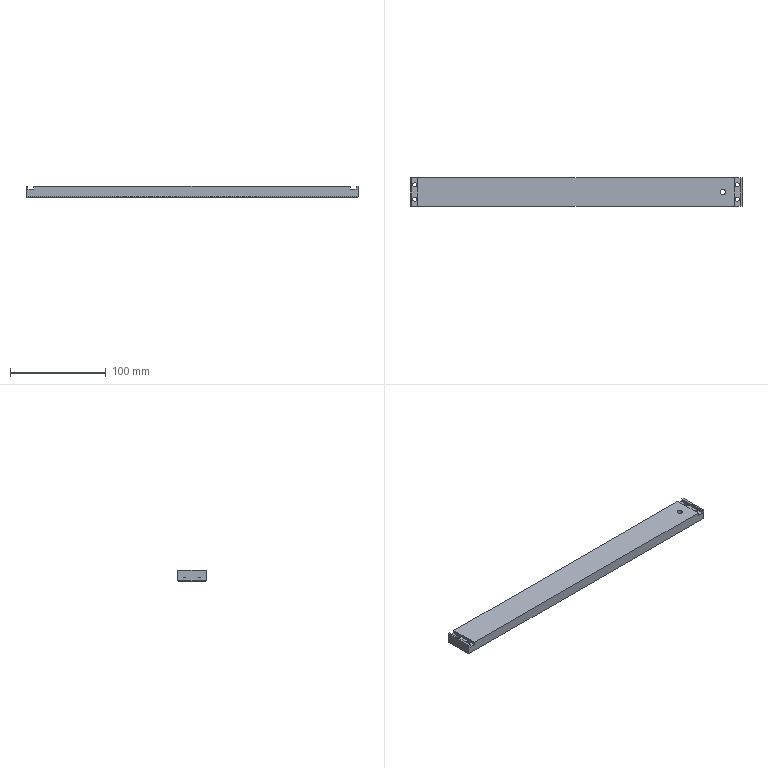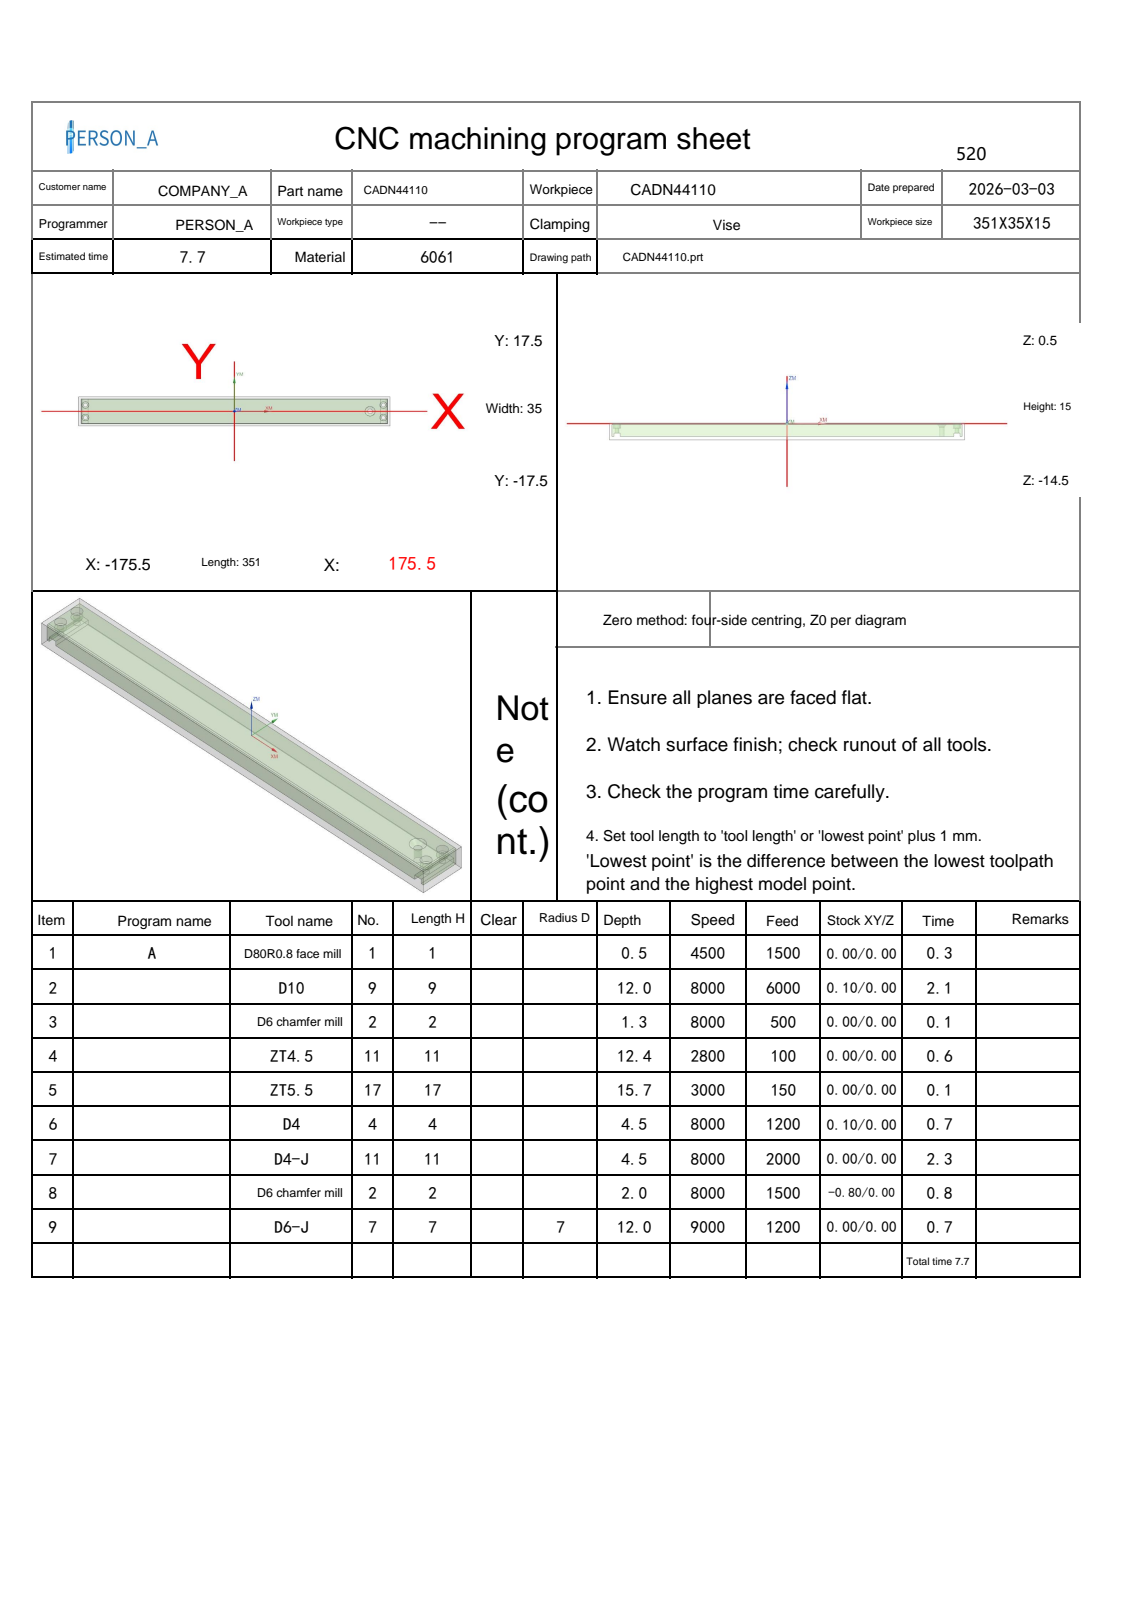NC program | NX | posted by the shop | part box 346 x 30 x 11.5 mm
Lines 337 to 1758 of 28539:
N7 T11 M06
(D4-J  D=4. R=0. H=11 ce=0.01 di=0.00)
G00 G90 G54 X149.305 Y-.481 M03 S7000
G43 H11 Z30.
M08
Z1.5
G01 X149.362 Y-.844 Z1.481 F2000.
X149.522 Y-1.359 Z1.452
X149.754 Y-1.846 Z1.424
X150.053 Y-2.294 Z1.396
X150.414 Y-2.695 Z1.368
X150.829 Y-3.039 Z1.339
X151.29 Y-3.32 Z1.311
X151.786 Y-3.531 Z1.283
X152.157 Y-3.638 Z1.263
X152.48 Y-3.698 Z1.245
X152.807 Y-3.729 Z1.228
X153.193 Z1.208
X153.206 Z1.207
X153.59 Y-3.687 Z1.187
X154.09 Y-3.572 Z1.16
X154.569 Y-3.389 Z1.133
X155.018 Y-3.142 Z1.106
X155.43 Y-2.836 Z1.08
X155.795 Y-2.477 Z1.053
X156.108 Y-2.07 Z1.026
X156.362 Y-1.625 Z.999
X156.553 Y-1.149 Z.972
X156.677 Y-.652 Z.945
X156.732 Y-.142 Z.918
X156.716 Y.37 Z.892
X156.63 Y.876 Z.865
X156.476 Y1.365 Z.838
X156.256 Y1.828 Z.811
X156.05 Y2.155 Z.791
X155.725 Y2.553 Z.764
X155.349 Y2.903 Z.737
X154.928 Y3.198 Z.71
X154.471 Y3.433 Z.683
X153.985 Y3.602 Z.656
X153.481 Y3.703 Z.629
X152.968 Y3.734 Z.602
X152.456 Y3.695 Z.575
X151.954 Y3.585 Z.548
X151.472 Y3.407 Z.521
X151.018 Y3.165 Z.494
X150.602 Y2.863 Z.467
X150.232 Y2.507 Z.44
X149.914 Y2.103 Z.414
X149.713 Y1.773 Z.393
X149.492 Y1.281 Z.365
X149.344 Y.762 Z.337
X149.273 Y.228 Z.309
X149.279 Y-.311 Z.28
X149.362 Y-.844 Z.252
X149.522 Y-1.359 Z.224
X149.754 Y-1.846 Z.195
X150.053 Y-2.294 Z.167
X150.414 Y-2.695 Z.139
X150.829 Y-3.039 Z.111
X151.29 Y-3.32 Z.082
X151.786 Y-3.531 Z.054
X152.157 Y-3.638 Z.034
X152.48 Y-3.698 Z.017
X152.807 Y-3.729 Z0.0
X153. Z-.011
G03 X156.729 Y0.0 I0.0 J3.729
X153. Y3.729 I-3.729 J0.0
X149.271 Y0.0 I0.0 J-3.729
X153. Y-3.729 I3.729 J0.0
G01 X153.1 Y-3.728
X153.199 Y-3.724
X153.3 Y-3.717
X153.399 Y-3.708
X153.586 Y-3.683
X153.771 Y-3.648
X153.955 Y-3.605
X154.137 Y-3.551
X154.315 Y-3.489
X154.49 Y-3.418
X154.661 Y-3.338
X154.828 Y-3.25
X154.99 Y-3.153 Z-.012
X155.147 Y-3.048
X155.299 Y-2.935
X155.445 Y-2.815
X155.584 Y-2.687
X155.717 Y-2.553
X155.843 Y-2.412
X155.961 Y-2.265
X156.072 Y-2.112
X156.175 Y-1.953
X156.27 Y-1.79
X156.356 Y-1.622 Z-.013
X156.434 Y-1.45
X156.503 Y-1.274
X156.563 Y-1.095
X156.614 Y-.913
X156.655 Y-.729
X156.687 Y-.543
X156.71 Y-.355
X156.723 Y-.167
X156.727 Y.022
X156.721 Y.211
X156.705 Y.399
X156.68 Y.586 Z-.014
X156.646 Y.772
X156.602 Y.955
X156.549 Y1.136
X156.486 Y1.315
X156.415 Y1.49
X156.335 Y1.661
X156.247 Y1.827
X156.15 Y1.99
X156.045 Y2.147
X155.932 Y2.299
X155.811 Y2.445
X155.684 Y2.584 Z-.015
X155.549 Y2.717
X155.408 Y2.843
X155.26 Y2.961
X155.107 Y3.072
X154.948 Y3.175
X154.784 Y3.27
X154.616 Y3.356
X154.443 Y3.434
X154.267 Y3.503
X154.088 Y3.562
X153.905 Y3.613 Z-.016
X153.721 Y3.654
X153.534 Y3.686
X153.346 Y3.708
X153.158 Y3.721
X152.968 Y3.724
X152.779 Y3.717
X152.591 Y3.701
X152.404 Y3.676
X152.218 Y3.641
X152.034 Y3.596
X151.853 Y3.542
X151.674 Y3.479 Z-.017
X151.499 Y3.408
X151.328 Y3.327
X151.162 Y3.238
X151. Y3.14
X150.843 Y3.034
X150.692 Y2.921
X150.546 Y2.8
X150.407 Y2.672
X150.275 Y2.536
X150.15 Y2.395
X150.032 Y2.247
X149.942 Y2.122 Z-.018
X149.856 Y1.993
X149.838 Y1.964
X149.82 Y1.934
X149.725 Y1.769
X149.639 Y1.6
X149.562 Y1.426
X149.494 Y1.249
X149.435 Y1.068
X149.385 Y.885
X149.345 Y.699
X149.314 Y.512
X149.292 Y.323
X149.281 Y.134 Z-.019
X149.279 Y-.056
X149.287 Y-.246
X149.304 Y-.435
X149.331 Y-.623
X149.368 Y-.81
X149.414 Y-.994
X149.47 Y-1.176
X149.534 Y-1.354
X149.608 Y-1.529
X149.691 Y-1.7
X149.782 Y-1.867
X149.881 Y-2.029 Z-.02
X149.989 Y-2.185
X150.104 Y-2.336
X150.227 Y-2.48
X150.358 Y-2.619
X150.495 Y-2.75
X150.638 Y-2.874
X150.788 Y-2.991
X150.944 Y-3.1
X151.105 Y-3.201
X151.27 Y-3.293
X151.441 Y-3.377
X151.615 Y-3.452 Z-.021
X151.793 Y-3.518
X151.974 Y-3.575
X151.992 Y-3.58
X152.01 Y-3.585
X152.16 Y-3.623
X152.311 Y-3.655
X152.482 Y-3.683
X152.654 Y-3.703
X152.827 Y-3.715
X153. Y-3.719
X153.1 Y-3.717
X153.199 Y-3.713
X153.3 Y-3.707
X153.399 Y-3.697
X153.586 Y-3.672
X153.771 Y-3.638 Z-.022
X153.954 Y-3.594
X154.135 Y-3.541
X154.313 Y-3.479
X154.488 Y-3.408
X154.658 Y-3.328
X154.825 Y-3.239
X154.987 Y-3.143
X155.143 Y-3.038
X155.295 Y-2.925
X155.44 Y-2.805
X155.579 Y-2.678 Z-.023
X155.711 Y-2.543
X155.837 Y-2.403
X155.955 Y-2.256
X156.065 Y-2.103
X156.168 Y-1.945
X156.262 Y-1.782
X156.348 Y-1.614
X156.426 Y-1.442
X156.494 Y-1.267
X156.554 Y-1.088
X156.604 Y-.906
X156.646 Y-.722 Z-.024
X156.677 Y-.537
X156.7 Y-.349
X156.713 Y-.161
X156.716 Y.027
X156.71 Y.215
X156.694 Y.403
X156.669 Y.59
X156.634 Y.775
X156.59 Y.958
X156.537 Y1.139
X156.474 Y1.317
X156.403 Y1.491 Z-.025
X156.323 Y1.662
X156.234 Y1.828
X156.138 Y1.99
X156.034 Y2.145
X155.922 Y2.294
X155.803 Y2.438
X155.677 Y2.576
X155.544 Y2.707
X155.404 Y2.832
X155.259 Y2.949
X155.108 Y3.059 Z-.026
X154.951 Y3.161
X154.79 Y3.255
X154.624 Y3.34
X154.454 Y3.418
X154.28 Y3.486
X154.104 Y3.546
X153.924 Y3.597
X153.742 Y3.639
X153.558 Y3.672
X153.373 Y3.695
X153.187 Y3.709
X153. Y3.713 Z-.027
X152.813 Y3.709
X152.627 Y3.695
X152.442 Y3.671
X152.258 Y3.638
X152.076 Y3.596
X151.897 Y3.545
X151.72 Y3.485
X151.546 Y3.416
X151.377 Y3.339
X151.211 Y3.253
X151.05 Y3.159
X150.893 Y3.057 Z-.028
X150.742 Y2.947
X150.597 Y2.83
X150.458 Y2.705
X150.325 Y2.574
X150.199 Y2.436
X150.081 Y2.293
X149.969 Y2.143
X149.865 Y1.988
X149.767 Y1.823
X149.677 Y1.653
X149.595 Y1.478
X149.524 Y1.3 Z-.029
X149.461 Y1.118
X149.408 Y.933
X149.364 Y.745
X149.331 Y.556
X149.307 Y.365
X149.293 Y.173
X149.289 Y-.019
X149.295 Y-.212
X149.311 Y-.403
X149.337 Y-.594
X149.373 Y-.783 Z-.03
X149.419 Y-.97
X149.474 Y-1.154
X149.538 Y-1.335
X149.612 Y-1.513
X149.695 Y-1.686
X149.787 Y-1.855
X149.888 Y-2.019
X149.997 Y-2.178
X150.114 Y-2.33
X150.238 Y-2.477
X150.371 Y-2.617
X150.51 Y-2.749 Z-.031
X150.656 Y-2.875
X150.808 Y-2.992
X150.966 Y-3.102
X151.129 Y-3.203
X151.298 Y-3.295
X151.471 Y-3.379
X151.648 Y-3.454
X151.829 Y-3.519
X152.013 Y-3.575
X152.032 Y-3.58
X152.051 Y-3.585
X152.194 Y-3.62
X152.338 Y-3.649 Z-.032
X152.502 Y-3.675
X152.668 Y-3.693
X152.834 Y-3.705
X153. Y-3.708
X153.1 Y-3.707
X153.199 Y-3.703
X153.3 Y-3.696
X153.399 Y-3.686
X153.585 Y-3.661
X153.77 Y-3.627
X153.953 Y-3.583
X154.133 Y-3.53
X154.311 Y-3.468
X154.485 Y-3.397 Z-.033
X154.655 Y-3.317
X154.822 Y-3.229
X154.983 Y-3.132
X155.139 Y-3.028
X155.29 Y-2.915
X155.435 Y-2.795
X155.574 Y-2.668
X155.706 Y-2.534
X155.831 Y-2.393
X155.948 Y-2.247
X156.058 Y-2.094
X156.161 Y-1.936 Z-.034
X156.255 Y-1.773
X156.34 Y-1.606
X156.417 Y-1.434
X156.486 Y-1.259
X156.545 Y-1.081
X156.595 Y-.899
X156.636 Y-.716
X156.668 Y-.53
X156.69 Y-.344
X156.702 Y-.156
X156.705 Y.032
X156.699 Y.22 Z-.035
X156.683 Y.407
X156.657 Y.594
X156.622 Y.778
X156.578 Y.961
X156.525 Y1.141
X156.462 Y1.319
X156.391 Y1.493
X156.311 Y1.663
X156.222 Y1.829
X156.125 Y1.99
X156.021 Y2.144 Z-.036
X155.91 Y2.293
X155.791 Y2.436
X155.665 Y2.573
X155.533 Y2.703
X155.394 Y2.827
X155.249 Y2.943
X155.098 Y3.052
X154.943 Y3.153
X154.782 Y3.247
X154.617 Y3.332
X154.447 Y3.409
X154.275 Y3.477 Z-.037
X154.099 Y3.537
X153.92 Y3.587
X153.739 Y3.629
X153.556 Y3.661
X153.371 Y3.684
X153.186 Y3.698
X153. Y3.703
X152.814 Y3.698
X152.629 Y3.684
X152.445 Y3.661
X152.262 Y3.628
X152.081 Y3.586 Z-.038
X151.902 Y3.536
X151.726 Y3.476
X151.553 Y3.408
X151.384 Y3.331
X151.219 Y3.245
X151.058 Y3.152
X150.903 Y3.05
X150.752 Y2.941
X150.608 Y2.825
X150.469 Y2.701
X150.337 Y2.571
X150.211 Y2.434 Z-.039
X150.093 Y2.291
X149.981 Y2.142
X149.878 Y1.988
X149.784 Y1.831
X149.697 Y1.67
X149.619 Y1.504
X149.548 Y1.335
X149.487 Y1.163
X149.434 Y.988
X149.389 Y.811
X149.354 Y.631
X149.327 Y.45 Z-.04
X149.309 Y.268
X149.301 Y.085
Y-.098
X149.311 Y-.28
X149.329 Y-.462
X149.356 Y-.643
X149.393 Y-.823
X149.438 Y-1.
X149.492 Y-1.175
X149.554 Y-1.347
X149.625 Y-1.515
X149.704 Y-1.68 Z-.041
X149.791 Y-1.841
X149.886 Y-1.997
X149.989 Y-2.149
X150.099 Y-2.295
X150.216 Y-2.435
X150.34 Y-2.57
X150.47 Y-2.698
X150.606 Y-2.82
X150.749 Y-2.935
X150.897 Y-3.042
X151.05 Y-3.142
X151.207 Y-3.235 Z-.042
X151.37 Y-3.32
X151.536 Y-3.396
X151.705 Y-3.464
X151.878 Y-3.524
X152.054 Y-3.575
X152.073 Y-3.58
X152.093 Y-3.585
X152.229 Y-3.617
X152.365 Y-3.643
X152.523 Y-3.667
X152.681 Y-3.684
X152.841 Y-3.694
X153. Y-3.698
X153.1 Y-3.696
X153.199 Y-3.692 Z-.043
X153.299 Y-3.685
X153.398 Y-3.676
X153.499 Y-3.664
X153.599 Y-3.648
X153.684 Y-3.633
X153.769 Y-3.616
X153.952 Y-3.573
X154.132 Y-3.52
X154.309 Y-3.458
X154.483 Y-3.387
X154.653 Y-3.307
X154.818 Y-3.219
X154.979 Y-3.122
X155.135 Y-3.017
X155.286 Y-2.905 Z-.044
X155.43 Y-2.785
X155.568 Y-2.658
X155.7 Y-2.524
X155.825 Y-2.384
X155.942 Y-2.237
X156.052 Y-2.085
X156.153 Y-1.927
X156.247 Y-1.765
X156.332 Y-1.598
X156.409 Y-1.426
X156.477 Y-1.251
X156.536 Y-1.073 Z-.045
X156.586 Y-.892
X156.627 Y-.709
X156.658 Y-.524
X156.68 Y-.338
X156.692 Y-.15
X156.695 Y.037
X156.688 Y.225
X156.672 Y.412
X156.646 Y.598
X156.611 Y.782
X156.566 Y.964 Z-.046
X156.513 Y1.144
X156.45 Y1.321
X156.379 Y1.494
X156.298 Y1.664
X156.209 Y1.829
X156.112 Y1.99
X156.009 Y2.143
X155.898 Y2.291
X155.779 Y2.433
X155.654 Y2.569
X155.522 Y2.699
X155.383 Y2.822 Z-.047
X155.239 Y2.937
X155.089 Y3.046
X154.934 Y3.146
X154.774 Y3.239
X154.609 Y3.324
X154.441 Y3.4
X154.269 Y3.468
X154.093 Y3.527
X153.915 Y3.577
X153.735 Y3.619
X153.553 Y3.651
X153.369 Y3.674 Z-.048
X153.185 Y3.688
X153. Y3.692
X152.815 Y3.688
X152.631 Y3.674
X152.447 Y3.65
X152.265 Y3.618
X152.085 Y3.577
X151.907 Y3.526
X151.732 Y3.467
X151.56 Y3.399
X151.391 Y3.323
X151.227 Y3.238 Z-.049
X151.067 Y3.145
X150.912 Y3.044
X150.762 Y2.936
X150.618 Y2.82
X150.48 Y2.697
X150.348 Y2.567
X150.223 Y2.431
X150.105 Y2.289
X149.994 Y2.141
X149.89 Y1.988
X149.795 Y1.83 Z-.05
X149.708 Y1.669
X149.63 Y1.503
X149.559 Y1.333
X149.497 Y1.16
X149.444 Y.984
X149.399 Y.806
X149.364 Y.626
X149.337 Y.444
X149.32 Y.261
X149.311 Y.078
X149.312 Y-.106
X149.322 Y-.289 Z-.051
X149.341 Y-.472
X149.369 Y-.653
X149.406 Y-.833
X149.452 Y-1.011
X149.507 Y-1.186
X149.57 Y-1.359
X149.642 Y-1.528
X149.722 Y-1.693
X149.811 Y-1.854
X149.907 Y-2.01
X150.011 Y-2.161
X150.122 Y-2.307 Z-.052
X150.241 Y-2.448
X150.366 Y-2.582
X150.498 Y-2.71
X150.636 Y-2.831
X150.78 Y-2.945
X150.929 Y-3.052
X151.084 Y-3.151
X151.243 Y-3.242
X151.406 Y-3.326
X151.574 Y-3.401
X151.745 Y-3.467
X151.919 Y-3.525 Z-.053
X152.096 Y-3.575
X152.117 Y-3.58
X152.138 Y-3.585
X152.265 Y-3.613
X152.394 Y-3.637
X152.544 Y-3.659
X152.696 Y-3.675
X152.848 Y-3.684
X153. Y-3.687
X153.15 Y-3.684
X153.3 Y-3.675
X153.45 Y-3.659
X153.599 Y-3.638
X153.787 Y-3.602
X153.972 Y-3.556
X154.156 Y-3.5 Z-.054
X154.337 Y-3.435
X154.514 Y-3.361
X154.686 Y-3.278
X154.855 Y-3.185
X155.018 Y-3.085
X155.176 Y-2.975
X155.328 Y-2.858
X155.473 Y-2.733
X155.612 Y-2.6
X155.744 Y-2.461
X155.868 Y-2.315 Z-.055
X155.984 Y-2.162
X156.093 Y-2.004
X156.193 Y-1.84
X156.284 Y-1.671
X156.367 Y-1.498
X156.44 Y-1.321
X156.504 Y-1.14
X156.559 Y-.956
X156.603 Y-.77
X156.638 Y-.581
X156.664 Y-.391 Z-.056
X156.679 Y-.2
X156.684 Y-.008
X156.68 Y.184
X156.665 Y.375
X156.64 Y.565
X156.606 Y.754
X156.562 Y.941
X156.508 Y1.125
X156.445 Y1.306
X156.372 Y1.483
X156.29 Y1.657
X156.199 Y1.826 Z-.057
X156.1 Y1.99
X155.996 Y2.142
X155.886 Y2.289
X155.767 Y2.43
X155.642 Y2.566
X155.511 Y2.694
X155.373 Y2.816
X155.229 Y2.932
X155.08 Y3.039
X154.925 Y3.139
X154.766 Y3.232
X154.602 Y3.316 Z-.058
X154.434 Y3.392
X154.263 Y3.459
X154.088 Y3.518
X153.911 Y3.568
X153.732 Y3.609
X153.55 Y3.641
X153.368 Y3.663
X153.184 Y3.677
X153. Y3.682
X152.816 Y3.677
X152.632 Y3.663 Z-.059
X152.45 Y3.64
X152.269 Y3.608
X152.089 Y3.567
X151.912 Y3.517
X151.738 Y3.458
X151.566 Y3.39
X151.399 Y3.314
X151.235 Y3.23
X151.076 Y3.138
X150.921 Y3.038
X150.772 Y2.93
X150.629 Y2.815 Z-.06
X150.491 Y2.693
X150.36 Y2.564
X150.235 Y2.428
X150.117 Y2.287
X150.006 Y2.14
X149.903 Y1.988
X149.807 Y1.83
X149.72 Y1.668
X149.64 Y1.501
X149.569 Y1.331
X149.507 Y1.157
X149.454 Y.981 Z-.061
X149.409 Y.802
X149.373 Y.621
X149.347 Y.438
X149.33 Y.254
X149.322 Y.07
X149.323 Y-.114
X149.333 Y-.298
X149.353 Y-.482
X149.382 Y-.664
X149.42 Y-.845
X149.467 Y-1.023
X149.522 Y-1.199 Z-.062
X149.587 Y-1.371
X149.66 Y-1.541
X149.741 Y-1.706
X149.831 Y-1.867
X149.929 Y-2.024
X150.034 Y-2.175
X150.147 Y-2.321
X150.267 Y-2.461
X150.394 Y-2.595
X150.527 Y-2.722
X150.667 Y-2.843
X150.812 Y-2.956 Z-.063
X150.963 Y-3.062
X151.119 Y-3.16
X151.28 Y-3.25
X151.445 Y-3.332
X151.614 Y-3.406
X151.786 Y-3.471
X151.962 Y-3.527
X152.14 Y-3.575
X152.162 Y-3.58
X152.184 Y-3.585
X152.304 Y-3.61
X152.424 Y-3.631
X152.567 Y-3.651
X152.711 Y-3.665 Z-.064
X152.855 Y-3.674
X153. Y-3.676
X153.15 Y-3.673
X153.3 Y-3.664
X153.45 Y-3.649
X153.599 Y-3.627
X153.786 Y-3.591
X153.971 Y-3.545
X154.155 Y-3.49
X154.335 Y-3.425
X154.511 Y-3.351
X154.684 Y-3.267
X154.852 Y-3.175 Z-.065
X155.014 Y-3.074
X155.172 Y-2.965
X155.323 Y-2.848
X155.468 Y-2.723
X155.607 Y-2.591
X155.738 Y-2.451
X155.862 Y-2.305
X155.978 Y-2.153
X156.086 Y-1.995
X156.186 Y-1.831
X156.277 Y-1.663 Z-.066
X156.359 Y-1.49
X156.432 Y-1.313
X156.495 Y-1.133
X156.549 Y-.949
X156.594 Y-.763
X156.629 Y-.575
X156.654 Y-.385
X156.669 Y-.194
X156.674 Y-.003
X156.669 Y.189
X156.654 Y.38
X156.629 Y.569 Z-.067
X156.594 Y.758
X156.55 Y.944
X156.496 Y1.127
X156.432 Y1.308
X156.36 Y1.485
X156.278 Y1.658
X156.187 Y1.826
X156.087 Y1.99
X155.984 Y2.141
X155.873 Y2.287
X155.756 Y2.428 Z-.068
X155.631 Y2.562
X155.5 Y2.69
X155.362 Y2.811
X155.219 Y2.926
X155.07 Y3.033
X154.916 Y3.132
X154.758 Y3.224
X154.595 Y3.307
X154.428 Y3.383
X154.257 Y3.45
X154.083 Y3.508
X153.907 Y3.558 Z-.069
X153.728 Y3.598
X153.548 Y3.63
X153.366 Y3.653
X153.183 Y3.667
X153. Y3.671
X152.817 Y3.666
X152.634 Y3.653
X152.452 Y3.63
X152.272 Y3.598
X152.093 Y3.557
X151.917 Y3.507
X151.743 Y3.449 Z-.07
X151.573 Y3.382
X151.406 Y3.306
X151.243 Y3.222
X151.085 Y3.131
X150.931 Y3.031
X150.782 Y2.924
X150.639 Y2.81
X150.502 Y2.688
X150.371 Y2.56
X150.247 Y2.426
X150.129 Y2.285
X150.019 Y2.139 Z-.071
X149.916 Y1.988
X149.819 Y1.829
X149.731 Y1.666
X149.651 Y1.499
X149.58 Y1.328
X149.517 Y1.154
X149.463 Y.976
X149.419 Y.797
X149.383 Y.615
X149.357 Y.431
X149.34 Y.247
X149.332 Y.062 Z-.072
X149.334 Y-.124
X149.345 Y-.309
X149.365 Y-.493
X149.395 Y-.676
X149.433 Y-.857
X149.481 Y-1.036
X149.538 Y-1.212
X149.604 Y-1.385
X149.678 Y-1.555
X149.761 Y-1.721
X149.852 Y-1.882 Z-.073
X149.951 Y-2.038
X150.058 Y-2.19
X150.173 Y-2.335
X150.294 Y-2.475
X150.423 Y-2.609
X150.558 Y-2.735
X150.699 Y-2.855
X150.846 Y-2.968
X150.999 Y-3.072
X151.156 Y-3.169
X151.319 Y-3.258
X151.486 Y-3.339 Z-.074
X151.656 Y-3.411
X151.83 Y-3.475
X152.007 Y-3.529
X152.187 Y-3.575
X152.21 Y-3.58
X152.233 Y-3.585
X152.344 Y-3.607
X152.455 Y-3.625
X152.591 Y-3.643
X152.727 Y-3.656
X152.863 Y-3.663
X153. Y-3.666
X153.15 Y-3.663
X153.3 Y-3.653
X153.45 Y-3.638
X153.599 Y-3.616 Z-.075
X153.786 Y-3.58
X153.971 Y-3.534
X154.153 Y-3.479
X154.333 Y-3.414
X154.509 Y-3.34
X154.681 Y-3.257
X154.849 Y-3.164
X155.011 Y-3.064
X155.168 Y-2.955
X155.319 Y-2.838
X155.464 Y-2.713
X155.602 Y-2.581 Z-.076
X155.732 Y-2.442
X155.856 Y-2.296
X155.972 Y-2.144
X156.079 Y-1.986
X156.178 Y-1.823
X156.269 Y-1.654
X156.351 Y-1.482
X156.423 Y-1.305
X156.487 Y-1.125
X156.54 Y-.942
X156.585 Y-.756 Z-.077
X156.619 Y-.568
X156.644 Y-.379
X156.658 Y-.188
X156.663 Y.003
X156.658 Y.194
X156.643 Y.384
X156.618 Y.573
X156.583 Y.761
X156.538 Y.947
X156.484 Y1.13
X156.42 Y1.31 Z-.078
X156.347 Y1.486
X156.265 Y1.659
X156.174 Y1.827
X156.075 Y1.99
X155.972 Y2.14
X155.861 Y2.285
X155.744 Y2.425
X155.62 Y2.559
X155.489 Y2.686
X155.352 Y2.806
X155.209 Y2.92
X155.061 Y3.026 Z-.079
X154.908 Y3.125
X154.75 Y3.216
X154.587 Y3.299
X154.421 Y3.374
X154.251 Y3.441
X154.078 Y3.499
X153.903 Y3.548
X153.725 Y3.588
X153.545 Y3.62
X153.364 Y3.642
X153.182 Y3.656
X153. Y3.66 Z-.08
X152.818 Y3.656
X152.636 Y3.642
X152.455 Y3.619
X152.275 Y3.588
X152.098 Y3.547
X151.922 Y3.498
X151.749 Y3.44
X151.58 Y3.373
X151.413 Y3.298
X151.251 Y3.215
X151.093 Y3.124
X150.94 Y3.025 Z-.081
X150.792 Y2.918
X150.65 Y2.805
X150.513 Y2.684
X150.382 Y2.557
X150.258 Y2.423
X150.141 Y2.284
X150.031 Y2.138
X149.928 Y1.988
X149.831 Y1.829
X149.742 Y1.665
X149.662 Y1.497
X149.59 Y1.325 Z-.082
X149.527 Y1.15
X149.473 Y.972
X149.428 Y.791
X149.393 Y.608
X149.367 Y.424
X149.35 Y.239
X149.343 Y.053
X149.345 Y-.134
X149.356 Y-.319
X149.377 Y-.504
X149.408 Y-.688 Z-.083
X149.448 Y-.87
X149.497 Y-1.05
X149.555 Y-1.227
X149.622 Y-1.4
X149.697 Y-1.57
X149.781 Y-1.736
X149.874 Y-1.898
X149.975 Y-2.054
X150.083 Y-2.206
X150.199 Y-2.351
X150.323 Y-2.49
X150.453 Y-2.623 Z-.084
X150.59 Y-2.75
X150.733 Y-2.869
X150.882 Y-2.98
X151.036 Y-3.084
X151.196 Y-3.18
X151.36 Y-3.267
X151.528 Y-3.347
X151.701 Y-3.417
X151.876 Y-3.479
X152.055 Y-3.531
X152.236 Y-3.575
X152.261 Y-3.58 Z-.085
X152.286 Y-3.585
X152.387 Y-3.604
X152.488 Y-3.619
X152.616 Y-3.635
X152.744 Y-3.646
X152.872 Y-3.653
X153. Y-3.655
X153.15 Y-3.652
X153.3 Y-3.643
X153.45 Y-3.627
X153.599 Y-3.605
X153.785 Y-3.569
X153.97 Y-3.524
X154.152 Y-3.468
X154.331 Y-3.403
X154.507 Y-3.329 Z-.086
X154.679 Y-3.246
X154.846 Y-3.154
X155.008 Y-3.053
X155.164 Y-2.944
X155.315 Y-2.827
X155.459 Y-2.703
X155.596 Y-2.571
X155.727 Y-2.432
X155.85 Y-2.286
X155.965 Y-2.134
X156.072 Y-1.977 Z-.087
X156.171 Y-1.814
X156.261 Y-1.646
X156.343 Y-1.474
X156.415 Y-1.297
X156.478 Y-1.117
X156.531 Y-.934
X156.575 Y-.749
X156.609 Y-.561
X156.634 Y-.372
X156.648 Y-.182
X156.652 Y.008 Z-.088
X156.647 Y.199
X156.632 Y.389
X156.606 Y.577
X156.571 Y.765
X156.526 Y.95
X156.472 Y1.133
X156.408 Y1.312
X156.335 Y1.488
X156.253 Y1.66
X156.162 Y1.827
X156.062 Y1.99
X155.959 Y2.139 Z-.089
X155.849 Y2.284
X155.732 Y2.422
X155.608 Y2.555
X155.478 Y2.682
X155.341 Y2.801
X155.199 Y2.914
X155.052 Y3.02
X154.899 Y3.118
X154.742 Y3.209
X154.58 Y3.291
X154.414 Y3.365
X154.245 Y3.431 Z-.09
X154.073 Y3.489
X153.898 Y3.538
X153.721 Y3.578
X153.543 Y3.61
X153.362 Y3.632
X153.181 Y3.645
X153. Y3.65
X152.819 Y3.645
X152.638 Y3.632
X152.458 Y3.609
X152.279 Y3.578
X152.102 Y3.537 Z-.091
X151.927 Y3.488
X151.755 Y3.43
X151.586 Y3.364
X151.421 Y3.29
X151.259 Y3.207
X151.102 Y3.116
X150.95 Y3.018
X150.802 Y2.912
X150.66 Y2.8
X150.524 Y2.68
X150.394 Y2.553 Z-.092
X150.27 Y2.42
X150.153 Y2.282
X150.043 Y2.137
X149.941 Y1.988
X149.843 Y1.828
X149.753 Y1.664
X149.672 Y1.495
X149.6 Y1.322
X149.537 Y1.146
X149.483 Y.967
X149.438 Y.785
X149.402 Y.601 Z-.093
X149.376 Y.416
X149.36 Y.229
X149.353 Y.042
X149.356 Y-.145
X149.368 Y-.332
X149.39 Y-.517
X149.421 Y-.702
X149.462 Y-.885
X149.512 Y-1.065
X149.572 Y-1.242
X149.64 Y-1.417
X149.717 Y-1.587 Z-.094
X149.803 Y-1.753
X149.897 Y-1.915
X150. Y-2.072
X150.11 Y-2.223
X150.228 Y-2.368
X150.353 Y-2.507
X150.485 Y-2.64
X150.624 Y-2.765
X150.769 Y-2.883
X150.92 Y-2.994
X151.076 Y-3.097 Z-.095
X151.238 Y-3.191
X151.404 Y-3.277
X151.574 Y-3.355
X151.748 Y-3.423
X151.925 Y-3.483
X152.105 Y-3.533
X152.288 Y-3.575
X152.315 Y-3.58
X152.342 Y-3.585
X152.492 Y-3.609
X152.642 Y-3.627
X152.821 Y-3.64
X153. Y-3.645
X153.15 Y-3.641 Z-.096
X153.3 Y-3.632
X153.449 Y-3.617
X153.598 Y-3.595
X153.784 Y-3.559
X153.969 Y-3.513
X154.151 Y-3.457
X154.33 Y-3.393
X154.505 Y-3.319
X154.676 Y-3.235
X154.843 Y-3.143
X155.004 Y-3.043
X155.16 Y-2.934 Z-.097
X155.31 Y-2.817
X155.454 Y-2.693
X155.591 Y-2.561
X155.721 Y-2.422
X155.844 Y-2.277
X155.959 Y-2.125
X156.066 Y-1.968
X156.164 Y-1.805
X156.254 Y-1.637
X156.335 Y-1.465
X156.407 Y-1.289 Z-.098
X156.469 Y-1.11
X156.522 Y-.927
X156.566 Y-.742
X156.6 Y-.555
X156.624 Y-.366
X156.638 Y-.177
X156.642 Y.014
X156.636 Y.204
X156.62 Y.393
X156.595 Y.582
X156.56 Y.768
X156.515 Y.953 Z-.099
X156.46 Y1.135
X156.396 Y1.314
X156.323 Y1.49
X156.24 Y1.661
X156.149 Y1.828
X156.049 Y1.99
X155.941 Y2.146
X155.825 Y2.297
X155.701 Y2.441
X155.57 Y2.579
X155.432 Y2.709 Z-.1
X155.287 Y2.832
X155.136 Y2.948
X154.979 Y3.055
X154.817 Y3.154
X154.649 Y3.245
X154.477 Y3.327
X154.302 Y3.399
X154.122 Y3.462
X153.94 Y3.516
X153.755 Y3.56
X153.568 Y3.595 Z-.101
X153.38 Y3.62
X153.19 Y3.634
X153. Y3.639
X152.81 Y3.634
X152.62 Y3.619
X152.432 Y3.594
X152.245 Y3.56
X152.06 Y3.515
X151.878 Y3.461
X151.699 Y3.398
X151.523 Y3.325
X151.351 Y3.244 Z-.102
X151.184 Y3.153
X151.022 Y3.054
X150.866 Y2.946
X150.715 Y2.831
X150.57 Y2.707
X150.432 Y2.577
X150.301 Y2.439
X150.177 Y2.295
X150.061 Y2.144
X149.954 Y1.988
X149.855 Y1.827 Z-.103
X149.765 Y1.662
X149.683 Y1.492
X149.61 Y1.319
X149.547 Y1.141
X149.492 Y.961
X149.447 Y.778
X149.412 Y.593
X149.386 Y.407
X149.37 Y.219
X149.364 Y.031
X149.367 Y-.157
X149.38 Y-.345 Z-.104
X149.403 Y-.532
X149.435 Y-.717
X149.477 Y-.901
X149.529 Y-1.082
X149.589 Y-1.26
X149.659 Y-1.435
X149.738 Y-1.606
X149.825 Y-1.772
X149.922 Y-1.934
X150.026 Y-2.091
X150.138 Y-2.242 Z-.105
X150.258 Y-2.387
X150.385 Y-2.526
X150.52 Y-2.657
X150.66 Y-2.782
X150.808 Y-2.899
X150.961 Y-3.009
X151.119 Y-3.11
X151.283 Y-3.203
X151.451 Y-3.288
X151.623 Y-3.364
X151.799 Y-3.43
X151.978 Y-3.488 Z-.106
X152.16 Y-3.536
X152.344 Y-3.575
X152.374 Y-3.58
X152.404 Y-3.585
X152.537 Y-3.605
X152.671 Y-3.619
X152.835 Y-3.63
X153. Y-3.634
X153.15 Y-3.631
X153.299 Y-3.621
X153.414 Y-3.61
X153.529 Y-3.595
X153.563 Y-3.59
X153.596 Y-3.584
X153.782 Y-3.548
X153.967 Y-3.503 Z-.107
X154.148 Y-3.447
X154.327 Y-3.382
X154.502 Y-3.308
X154.672 Y-3.225
X154.839 Y-3.133
X155. Y-3.033
X155.155 Y-2.924
X155.305 Y-2.808
X155.449 Y-2.683
X155.585 Y-2.552
X155.715 Y-2.413
X155.837 Y-2.268 Z-.108
X155.952 Y-2.117
X156.058 Y-1.959
X156.156 Y-1.797
X156.246 Y-1.63
X156.327 Y-1.458
X156.398 Y-1.282
X156.46 Y-1.103
X156.513 Y-.92
X156.556 Y-.736
X156.59 Y-.549
X156.614 Y-.36 Z-.109
X156.627 Y-.171
X156.631 Y.019
X156.625 Y.208
X156.609 Y.397
X156.584 Y.585
X156.548 Y.772
X156.503 Y.956
X156.448 Y1.138
X156.384 Y1.316
X156.31 Y1.491
X156.228 Y1.662 Z-.11
X156.136 Y1.828
X156.037 Y1.99
X155.929 Y2.145
X155.813 Y2.295
X155.689 Y2.438
X155.559 Y2.575
X155.421 Y2.705
X155.276 Y2.827
X155.126 Y2.942
X154.97 Y3.049
X154.808 Y3.147
X154.642 Y3.237 Z-.111
X154.471 Y3.318
X154.296 Y3.39
X154.117 Y3.453
X153.936 Y3.506
X153.751 Y3.55
X153.565 Y3.585
X153.378 Y3.609
X153.189 Y3.624
X153. Y3.629
X152.811 Y3.624
X152.622 Y3.609 Z-.112
X152.435 Y3.584
X152.249 Y3.55
X152.065 Y3.506
X151.883 Y3.452
X151.705 Y3.389
X151.53 Y3.317
X151.359 Y3.236
X151.193 Y3.146
X151.031 Y3.047
X150.875 Y2.94
X150.725 Y2.825 Z-.113
X150.581 Y2.703
X150.443 Y2.573
X150.313 Y2.436
X150.189 Y2.293
X150.074 Y2.143
X149.966 Y1.988
X149.867 Y1.826
X149.776 Y1.66
X149.693 Y1.489
X149.62 Y1.315
X149.556 Y1.136
X149.502 Y.955 Z-.114
X149.457 Y.771
X149.421 Y.585
X149.396 Y.397
X149.38 Y.208
X149.374 Y.019
X149.378 Y-.171
X149.392 Y-.36
X149.416 Y-.548
X149.45 Y-.734
X149.493 Y-.919
X149.546 Y-1.101 Z-.115
X149.608 Y-1.28
X149.68 Y-1.455
X149.76 Y-1.627
X149.85 Y-1.793
X149.948 Y-1.956
X150.054 Y-2.112
X150.169 Y-2.263
X150.291 Y-2.408
X150.42 Y-2.546
X150.557 Y-2.677
X150.7 Y-2.801 Z-.116
X150.85 Y-2.918
X151.005 Y-3.026
X151.166 Y-3.126
X151.332 Y-3.217
X151.502 Y-3.3
X151.677 Y-3.374
X151.855 Y-3.438
X152.036 Y-3.493
X152.22 Y-3.539
X152.406 Y-3.575
X152.439 Y-3.58
X152.472 Y-3.585
X152.587 Y-3.6
X152.702 Y-3.611 Z-.117
X152.851 Y-3.62
X153. Y-3.623
X153.132 Y-3.621
X153.264 Y-3.614
X153.357 Y-3.605
X153.45 Y-3.595
X153.489 Y-3.59
X153.528 Y-3.584
X153.707 Y-3.553
X153.884 Y-3.513
X154.059 Y-3.465
X154.231 Y-3.407
X154.401 Y-3.341
X154.566 Y-3.266
X154.728 Y-3.184 Z-.118
X154.885 Y-3.093
X155.038 Y-2.995
X155.186 Y-2.888
X155.328 Y-2.775
X155.464 Y-2.655
X155.594 Y-2.528
X155.717 Y-2.395
X155.834 Y-2.255
X155.943 Y-2.11
X156.045 Y-1.96
X156.14 Y-1.805
X156.226 Y-1.645 Z-.119
X156.305 Y-1.481
X156.375 Y-1.314
X156.436 Y-1.143
X156.489 Y-.969
X156.533 Y-.793
X156.568 Y-.615
X156.595 Y-.435
X156.612 Y-.254
X156.62 Y-.073
X156.619 Y.109
X156.609 Y.29
X156.59 Y.471 Z-.12
X156.561 Y.65
X156.524 Y.828
X156.478 Y1.004
X156.423 Y1.177
X156.36 Y1.347
X156.288 Y1.514
X156.208 Y1.677
X156.118 Y1.838
X156.02 Y1.995
X155.914 Y2.147
X155.801 Y2.293
X155.678 Y2.435 Z-.121
X155.547 Y2.571
X155.41 Y2.7
X155.266 Y2.822
X155.116 Y2.936
X154.961 Y3.042
X154.8 Y3.14
X154.634 Y3.229
X154.464 Y3.31
X154.289 Y3.381
X154.112 Y3.444
X153.931 Y3.497 Z-.122
X153.748 Y3.54
X153.563 Y3.574
X153.376 Y3.599
X153.188 Y3.613
X153. Y3.618
X152.812 Y3.613
X152.624 Y3.598
X152.437 Y3.574
X152.252 Y3.54
X152.069 Y3.496
X151.889 Y3.443 Z-.123
X151.711 Y3.38